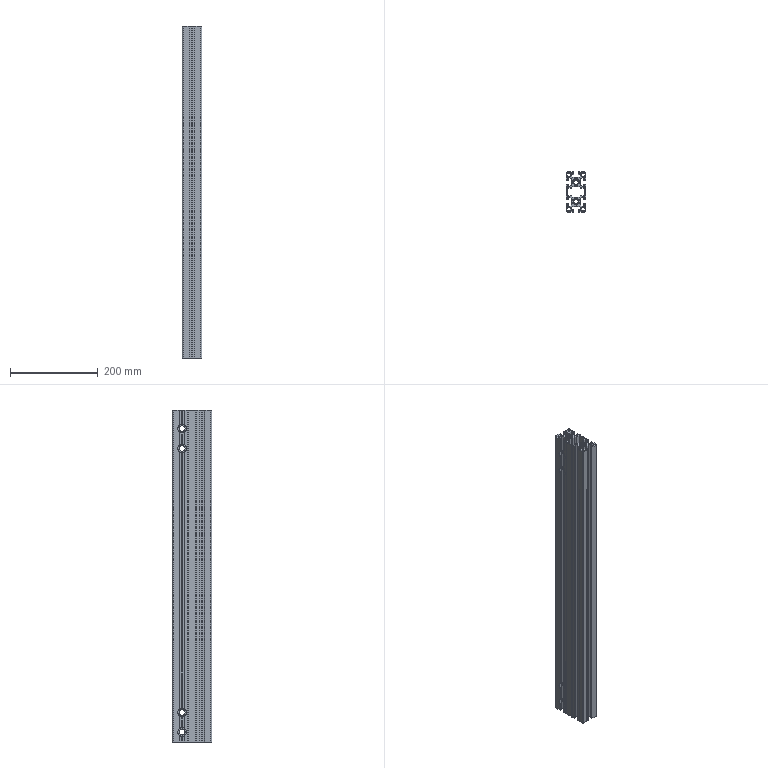Part | STEP file | PN_0014 | 1 solid | 992 faces | box 45 x 90 x 757.5 mm | volume 975869 mm3 | cylinder 610 | plane 382 | commonest cylinder face diameters 1 x260 0.6 x120 2 x56 10.2 x54 16 x32 20 x32